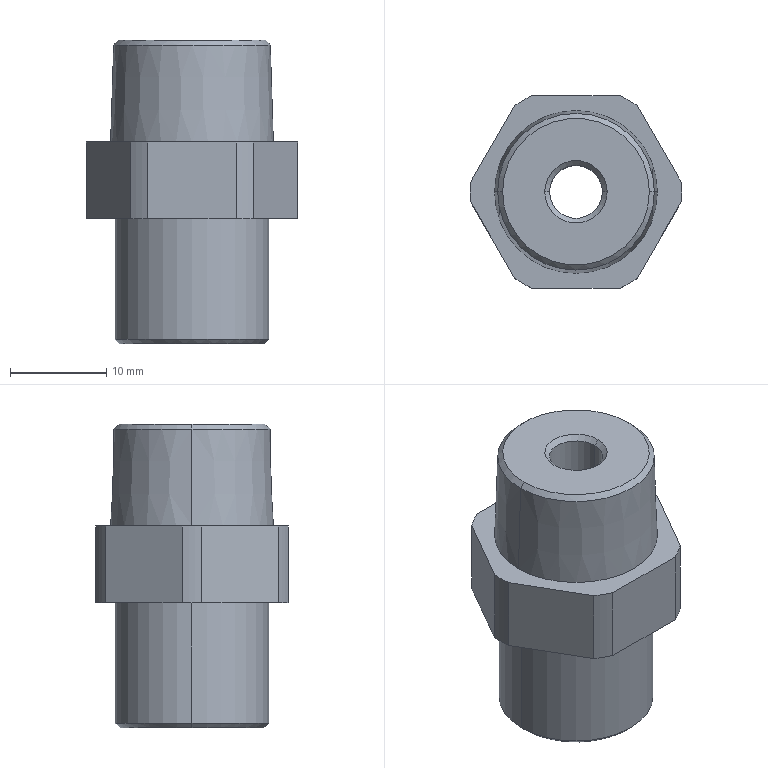Part | STEP file | HXGR200008-06-03-03 | 1 solid | 31 faces | box 22 x 20 x 31.6 mm | volume 6624 mm3 | cylinder 11 | cone 10 | plane 10 | commonest cylinder face diameters 22 x7 5.5 x2 16 x2
STEP:
#1=CARTESIAN_POINT('',(10.952,-1.031,0.));
#2=VERTEX_POINT('',#1);
#3=CARTESIAN_POINT('',(11.,0.,0.));
#4=VERTEX_POINT('',#3);
#5=CARTESIAN_POINT('',(0.,0.,0.));
#6=DIRECTION('',(0.,0.,1.));
#7=DIRECTION('',(1.,0.,0.));
#8=AXIS2_PLACEMENT_3D('',#5,#6,#7);
#9=CIRCLE('',#8,11.);
#10=EDGE_CURVE('',#2,#4,#9,.T.);
#11=ORIENTED_EDGE('',*,*,#10,.T.);
#12=CARTESIAN_POINT('',(11.,0.,8.));
#13=VERTEX_POINT('',#12);
#14=CARTESIAN_POINT('',(11.,0.,-13.));
#15=DIRECTION('',(0.,0.,1.));
#16=VECTOR('',#15,1000.);
#17=LINE('',#14,#16);
#18=EDGE_CURVE('',#4,#13,#17,.T.);
#19=ORIENTED_EDGE('',*,*,#18,.T.);
#20=CARTESIAN_POINT('',(10.952,-1.031,8.));
#21=VERTEX_POINT('',#20);
#22=CARTESIAN_POINT('',(0.,0.,8.));
#23=DIRECTION('',(0.,0.,1.));
#24=DIRECTION('',(1.,0.,0.));
#25=AXIS2_PLACEMENT_3D('',#22,#23,#24);
#26=CIRCLE('',#25,11.);
#27=EDGE_CURVE('',#21,#13,#26,.T.);
#28=ORIENTED_EDGE('',*,*,#27,.F.);
#29=CARTESIAN_POINT('',(10.952,-1.031,-13.));
#30=DIRECTION('',(0.,0.,-1.));
#31=VECTOR('',#30,1000.);
#32=LINE('',#29,#31);
#33=EDGE_CURVE('',#21,#2,#32,.T.);
#34=ORIENTED_EDGE('',*,*,#33,.T.);
#35=EDGE_LOOP('',(#11,#19,#28,#34));
#36=FACE_OUTER_BOUND('',#35,.T.);
#37=CARTESIAN_POINT('',(0.,0.,-13.));
#38=DIRECTION('',(0.,0.,1.));
#39=DIRECTION('',(1.,0.,0.));
#40=AXIS2_PLACEMENT_3D('',#37,#38,#39);
#41=CYLINDRICAL_SURFACE('',#40,11.);
#42=ADVANCED_FACE('',(#36),#41,.T.);
#43=CARTESIAN_POINT('',(-7.5,0.,-13.));
#44=VERTEX_POINT('',#43);
#45=CARTESIAN_POINT('',(7.5,0.,-13.));
#46=VERTEX_POINT('',#45);
#47=CARTESIAN_POINT('',(0.,0.,-13.));
#48=DIRECTION('',(0.,0.,-1.));
#49=DIRECTION('',(-1.,0.,0.));
#50=AXIS2_PLACEMENT_3D('',#47,#48,#49);
#51=CIRCLE('',#50,7.5);
#52=EDGE_CURVE('',#44,#46,#51,.T.);
#53=ORIENTED_EDGE('',*,*,#52,.F.);
#54=CARTESIAN_POINT('',(-8.,0.,-12.5));
#55=VERTEX_POINT('',#54);
#56=CARTESIAN_POINT('',(-7.5,0.,-13.));
#57=DIRECTION('',(-0.7071,0.,0.7071));
#58=VECTOR('',#57,1000.);
#59=LINE('',#56,#58);
#60=EDGE_CURVE('',#44,#55,#59,.T.);
#61=ORIENTED_EDGE('',*,*,#60,.T.);
#62=CARTESIAN_POINT('',(8.,0.,-12.5));
#63=VERTEX_POINT('',#62);
#64=CARTESIAN_POINT('',(0.,0.,-12.5));
#65=DIRECTION('',(0.,0.,1.));
#66=DIRECTION('',(-1.,0.,0.));
#67=AXIS2_PLACEMENT_3D('',#64,#65,#66);
#68=CIRCLE('',#67,8.);
#69=EDGE_CURVE('',#63,#55,#68,.T.);
#70=ORIENTED_EDGE('',*,*,#69,.F.);
#71=CARTESIAN_POINT('',(7.5,0.,-13.));
#72=DIRECTION('',(0.7071,0.,0.7071));
#73=VECTOR('',#72,1000.);
#74=LINE('',#71,#73);
#75=EDGE_CURVE('',#46,#63,#74,.T.);
#76=ORIENTED_EDGE('',*,*,#75,.F.);
#77=EDGE_LOOP('',(#53,#61,#70,#76));
#78=FACE_OUTER_BOUND('',#77,.T.);
#79=CARTESIAN_POINT('',(0.,0.,-13.));
#80=DIRECTION('',(0.,0.,1.));
#81=DIRECTION('',(1.,0.,0.));
#82=AXIS2_PLACEMENT_3D('',#79,#80,#81);
#83=CONICAL_SURFACE('',#82,7.5,0.7854);
#84=ADVANCED_FACE('',(#78),#83,.T.);
#85=CARTESIAN_POINT('',(7.63,0.,18.6));
#86=VERTEX_POINT('',#85);
#87=CARTESIAN_POINT('',(-7.63,0.,18.6));
#88=VERTEX_POINT('',#87);
#89=CARTESIAN_POINT('',(0.,0.,18.6));
#90=DIRECTION('',(0.,0.,1.));
#91=DIRECTION('',(1.,0.,0.));
#92=AXIS2_PLACEMENT_3D('',#89,#90,#91);
#93=CIRCLE('',#92,7.63);
#94=EDGE_CURVE('',#86,#88,#93,.T.);
#95=ORIENTED_EDGE('',*,*,#94,.F.);
#96=CARTESIAN_POINT('',(8.146,0.,18.084));
#97=VERTEX_POINT('',#96);
#98=CARTESIAN_POINT('',(8.146,0.,18.084));
#99=DIRECTION('',(0.7071,0.,-0.7071));
#100=VECTOR('',#99,1000.);
#101=LINE('',#98,#100);
#102=EDGE_CURVE('',#86,#97,#101,.T.);
#103=ORIENTED_EDGE('',*,*,#102,.T.);
#104=CARTESIAN_POINT('',(-8.146,0.,18.084));
#105=VERTEX_POINT('',#104);
#106=CARTESIAN_POINT('',(0.,0.,18.084));
#107=DIRECTION('',(0.,0.,-1.));
#108=DIRECTION('',(1.,0.,0.));
#109=AXIS2_PLACEMENT_3D('',#106,#107,#108);
#110=CIRCLE('',#109,8.146);
#111=EDGE_CURVE('',#105,#97,#110,.T.);
#112=ORIENTED_EDGE('',*,*,#111,.F.);
#113=CARTESIAN_POINT('',(-8.146,0.,18.084));
#114=DIRECTION('',(-0.7071,0.,-0.7071));
#115=VECTOR('',#114,1000.);
#116=LINE('',#113,#115);
#117=EDGE_CURVE('',#88,#105,#116,.T.);
#118=ORIENTED_EDGE('',*,*,#117,.F.);
#119=EDGE_LOOP('',(#95,#103,#112,#118));
#120=FACE_OUTER_BOUND('',#119,.T.);
#121=CARTESIAN_POINT('',(0.,0.,18.084));
#122=DIRECTION('',(0.,0.,-1.));
#123=DIRECTION('',(-1.,0.,0.));
#124=AXIS2_PLACEMENT_3D('',#121,#122,#123);
#125=CONICAL_SURFACE('',#124,8.146,0.7854);
#126=ADVANCED_FACE('',(#120),#125,.T.);
#127=CARTESIAN_POINT('',(-2.75,0.,18.1));
#128=VERTEX_POINT('',#127);
#129=CARTESIAN_POINT('',(2.75,0.,18.1));
#130=VERTEX_POINT('',#129);
#131=CARTESIAN_POINT('',(0.,0.,18.1));
#132=DIRECTION('',(0.,0.,1.));
#133=DIRECTION('',(1.,0.,0.));
#134=AXIS2_PLACEMENT_3D('',#131,#132,#133);
#135=CIRCLE('',#134,2.75);
#136=EDGE_CURVE('',#128,#130,#135,.T.);
#137=ORIENTED_EDGE('',*,*,#136,.F.);
#138=CARTESIAN_POINT('',(-3.25,0.,18.6));
#139=VERTEX_POINT('',#138);
#140=CARTESIAN_POINT('',(-2.75,0.,18.1));
#141=DIRECTION('',(-0.7071,0.,0.7071));
#142=VECTOR('',#141,1000.);
#143=LINE('',#140,#142);
#144=EDGE_CURVE('',#128,#139,#143,.T.);
#145=ORIENTED_EDGE('',*,*,#144,.T.);
#146=CARTESIAN_POINT('',(3.25,0.,18.6));
#147=VERTEX_POINT('',#146);
#148=CARTESIAN_POINT('',(0.,0.,18.6));
#149=DIRECTION('',(0.,0.,-1.));
#150=DIRECTION('',(1.,0.,0.));
#151=AXIS2_PLACEMENT_3D('',#148,#149,#150);
#152=CIRCLE('',#151,3.25);
#153=EDGE_CURVE('',#147,#139,#152,.T.);
#154=ORIENTED_EDGE('',*,*,#153,.F.);
#155=CARTESIAN_POINT('',(2.75,0.,18.1));
#156=DIRECTION('',(0.7071,0.,0.7071));
#157=VECTOR('',#156,1000.);
#158=LINE('',#155,#157);
#159=EDGE_CURVE('',#130,#147,#158,.T.);
#160=ORIENTED_EDGE('',*,*,#159,.F.);
#161=EDGE_LOOP('',(#137,#145,#154,#160));
#162=FACE_OUTER_BOUND('',#161,.T.);
#163=CARTESIAN_POINT('',(0.,0.,18.1));
#164=DIRECTION('',(0.,0.,1.));
#165=DIRECTION('',(1.,0.,0.));
#166=AXIS2_PLACEMENT_3D('',#163,#164,#165);
#167=CONICAL_SURFACE('',#166,2.75,0.7854);
#168=ADVANCED_FACE('',(#162),#167,.F.);
#169=CARTESIAN_POINT('',(2.75,0.,-6.938));
#170=VERTEX_POINT('',#169);
#171=CARTESIAN_POINT('',(-2.75,0.,-6.938));
#172=VERTEX_POINT('',#171);
#173=CARTESIAN_POINT('',(0.,0.,-6.938));
#174=DIRECTION('',(0.,0.,-1.));
#175=DIRECTION('',(-1.,0.,0.));
#176=AXIS2_PLACEMENT_3D('',#173,#174,#175);
#177=CIRCLE('',#176,2.75);
#178=EDGE_CURVE('',#170,#172,#177,.T.);
#179=ORIENTED_EDGE('',*,*,#178,.F.);
#180=CARTESIAN_POINT('',(6.25,0.,-13.));
#181=VERTEX_POINT('',#180);
#182=CARTESIAN_POINT('',(6.25,0.,-13.));
#183=DIRECTION('',(0.5,0.,-0.866));
#184=VECTOR('',#183,1000.);
#185=LINE('',#182,#184);
#186=EDGE_CURVE('',#170,#181,#185,.T.);
#187=ORIENTED_EDGE('',*,*,#186,.T.);
#188=CARTESIAN_POINT('',(-6.25,0.,-13.));
#189=VERTEX_POINT('',#188);
#190=CARTESIAN_POINT('',(0.,0.,-13.));
#191=DIRECTION('',(0.,0.,-1.));
#192=DIRECTION('',(-1.,0.,0.));
#193=AXIS2_PLACEMENT_3D('',#190,#191,#192);
#194=CIRCLE('',#193,6.25);
#195=EDGE_CURVE('',#181,#189,#194,.T.);
#196=ORIENTED_EDGE('',*,*,#195,.T.);
#197=CARTESIAN_POINT('',(-6.25,0.,-13.));
#198=DIRECTION('',(-0.5,0.,-0.866));
#199=VECTOR('',#198,1000.);
#200=LINE('',#197,#199);
#201=EDGE_CURVE('',#172,#189,#200,.T.);
#202=ORIENTED_EDGE('',*,*,#201,.F.);
#203=EDGE_LOOP('',(#179,#187,#196,#202));
#204=FACE_OUTER_BOUND('',#203,.T.);
#205=CARTESIAN_POINT('',(0.,0.,-13.));
#206=DIRECTION('',(0.,0.,-1.));
#207=DIRECTION('',(-1.,0.,0.));
#208=AXIS2_PLACEMENT_3D('',#205,#206,#207);
#209=CONICAL_SURFACE('',#208,6.25,0.5236);
#210=ADVANCED_FACE('',(#204),#209,.F.);
#211=ORIENTED_EDGE('',*,*,#178,.T.);
#212=CARTESIAN_POINT('',(-2.75,0.,-13.001));
#213=DIRECTION('',(0.,0.,1.));
#214=VECTOR('',#213,1000.);
#215=LINE('',#212,#214);
#216=EDGE_CURVE('',#172,#128,#215,.T.);
#217=ORIENTED_EDGE('',*,*,#216,.T.);
#218=ORIENTED_EDGE('',*,*,#136,.T.);
#219=CARTESIAN_POINT('',(2.75,0.,-13.001));
#220=DIRECTION('',(0.,0.,1.));
#221=VECTOR('',#220,1000.);
#222=LINE('',#219,#221);
#223=EDGE_CURVE('',#170,#130,#222,.T.);
#224=ORIENTED_EDGE('',*,*,#223,.F.);
#225=EDGE_LOOP('',(#211,#217,#218,#224));
#226=FACE_OUTER_BOUND('',#225,.T.);
#227=CARTESIAN_POINT('',(0.,0.,-13.001));
#228=DIRECTION('',(0.,0.,1.));
#229=DIRECTION('',(1.,0.,0.));
#230=AXIS2_PLACEMENT_3D('',#227,#228,#229);
#231=CYLINDRICAL_SURFACE('',#230,2.75);
#232=ADVANCED_FACE('',(#226),#231,.F.);
#233=ORIENTED_EDGE('',*,*,#111,.T.);
#234=CARTESIAN_POINT('',(8.46,0.,8.));
#235=VERTEX_POINT('',#234);
#236=CARTESIAN_POINT('',(8.46,0.,8.));
#237=DIRECTION('',(0.03112,0.,-0.9995));
#238=VECTOR('',#237,1000.);
#239=LINE('',#236,#238);
#240=EDGE_CURVE('',#97,#235,#239,.T.);
#241=ORIENTED_EDGE('',*,*,#240,.T.);
#242=CARTESIAN_POINT('',(-8.46,0.,8.));
#243=VERTEX_POINT('',#242);
#244=CARTESIAN_POINT('',(0.,0.,8.));
#245=DIRECTION('',(0.,0.,-1.));
#246=DIRECTION('',(-1.,0.,0.));
#247=AXIS2_PLACEMENT_3D('',#244,#245,#246);
#248=CIRCLE('',#247,8.46);
#249=EDGE_CURVE('',#243,#235,#248,.T.);
#250=ORIENTED_EDGE('',*,*,#249,.F.);
#251=CARTESIAN_POINT('',(-8.46,0.,8.));
#252=DIRECTION('',(-0.03112,0.,-0.9995));
#253=VECTOR('',#252,1000.);
#254=LINE('',#251,#253);
#255=EDGE_CURVE('',#105,#243,#254,.T.);
#256=ORIENTED_EDGE('',*,*,#255,.F.);
#257=EDGE_LOOP('',(#233,#241,#250,#256));
#258=FACE_OUTER_BOUND('',#257,.T.);
#259=CARTESIAN_POINT('',(0.,0.,8.));
#260=DIRECTION('',(0.,0.,-1.));
#261=DIRECTION('',(-1.,0.,0.));
#262=AXIS2_PLACEMENT_3D('',#259,#260,#261);
#263=CONICAL_SURFACE('',#262,8.46,0.03112);
#264=ADVANCED_FACE('',(#258),#263,.T.);
#265=ORIENTED_EDGE('',*,*,#69,.T.);
#266=CARTESIAN_POINT('',(-8.,0.,0.));
#267=VERTEX_POINT('',#266);
#268=CARTESIAN_POINT('',(-8.,0.,-13.));
#269=DIRECTION('',(0.,0.,1.));
#270=VECTOR('',#269,1000.);
#271=LINE('',#268,#270);
#272=EDGE_CURVE('',#55,#267,#271,.T.);
#273=ORIENTED_EDGE('',*,*,#272,.T.);
#274=CARTESIAN_POINT('',(8.,0.,0.));
#275=VERTEX_POINT('',#274);
#276=CARTESIAN_POINT('',(0.,0.,0.));
#277=DIRECTION('',(0.,0.,-1.));
#278=DIRECTION('',(-1.,0.,0.));
#279=AXIS2_PLACEMENT_3D('',#276,#277,#278);
#280=CIRCLE('',#279,8.);
#281=EDGE_CURVE('',#267,#275,#280,.T.);
#282=ORIENTED_EDGE('',*,*,#281,.T.);
#283=CARTESIAN_POINT('',(8.,0.,-13.));
#284=DIRECTION('',(0.,0.,1.));
#285=VECTOR('',#284,1000.);
#286=LINE('',#283,#285);
#287=EDGE_CURVE('',#63,#275,#286,.T.);
#288=ORIENTED_EDGE('',*,*,#287,.F.);
#289=EDGE_LOOP('',(#265,#273,#282,#288));
#290=FACE_OUTER_BOUND('',#289,.T.);
#291=CARTESIAN_POINT('',(0.,0.,-13.));
#292=DIRECTION('',(0.,0.,1.));
#293=DIRECTION('',(1.,0.,0.));
#294=AXIS2_PLACEMENT_3D('',#291,#292,#293);
#295=CYLINDRICAL_SURFACE('',#294,8.);
#296=ADVANCED_FACE('',(#290),#295,.T.);
#297=CARTESIAN_POINT('',(6.369,-8.969,0.));
#298=VERTEX_POINT('',#297);
#299=CARTESIAN_POINT('',(6.369,-8.969,8.));
#300=VERTEX_POINT('',#299);
#301=CARTESIAN_POINT('',(6.369,-8.969,-13.));
#302=DIRECTION('',(0.,0.,1.));
#303=VECTOR('',#302,1000.);
#304=LINE('',#301,#303);
#305=EDGE_CURVE('',#298,#300,#304,.T.);
#306=ORIENTED_EDGE('',*,*,#305,.F.);
#307=CARTESIAN_POINT('',(5.774,-10.,0.));
#308=DIRECTION('',(0.5,0.866,0.));
#309=VECTOR('',#308,1000.);
#310=LINE('',#307,#309);
#311=EDGE_CURVE('',#298,#2,#310,.T.);
#312=ORIENTED_EDGE('',*,*,#311,.T.);
#313=ORIENTED_EDGE('',*,*,#33,.F.);
#314=CARTESIAN_POINT('',(5.774,-10.,8.));
#315=DIRECTION('',(0.5,0.866,0.));
#316=VECTOR('',#315,1000.);
#317=LINE('',#314,#316);
#318=EDGE_CURVE('',#300,#21,#317,.T.);
#319=ORIENTED_EDGE('',*,*,#318,.F.);
#320=EDGE_LOOP('',(#306,#312,#313,#319));
#321=FACE_OUTER_BOUND('',#320,.T.);
#322=CARTESIAN_POINT('',(5.774,-10.,8.));
#323=DIRECTION('',(-0.866,0.5,0.));
#324=DIRECTION('',(-0.5,-0.866,0.));
#325=AXIS2_PLACEMENT_3D('',#322,#323,#324);
#326=PLANE('',#325);
#327=ADVANCED_FACE('',(#321),#326,.F.);
#328=CARTESIAN_POINT('',(10.952,1.031,0.));
#329=VERTEX_POINT('',#328);
#330=CARTESIAN_POINT('',(10.952,1.031,8.));
#331=VERTEX_POINT('',#330);
#332=CARTESIAN_POINT('',(10.952,1.031,-13.));
#333=DIRECTION('',(0.,0.,1.));
#334=VECTOR('',#333,1000.);
#335=LINE('',#332,#334);
#336=EDGE_CURVE('',#329,#331,#335,.T.);
#337=ORIENTED_EDGE('',*,*,#336,.F.);
#338=CARTESIAN_POINT('',(6.369,8.969,0.));
#339=VERTEX_POINT('',#338);
#340=CARTESIAN_POINT('',(11.547,0.,0.));
#341=DIRECTION('',(-0.5,0.866,0.));
#342=VECTOR('',#341,1000.);
#343=LINE('',#340,#342);
#344=EDGE_CURVE('',#329,#339,#343,.T.);
#345=ORIENTED_EDGE('',*,*,#344,.T.);
#346=CARTESIAN_POINT('',(6.369,8.969,8.));
#347=VERTEX_POINT('',#346);
#348=CARTESIAN_POINT('',(6.369,8.969,-13.));
#349=DIRECTION('',(0.,0.,-1.));
#350=VECTOR('',#349,1000.);
#351=LINE('',#348,#350);
#352=EDGE_CURVE('',#347,#339,#351,.T.);
#353=ORIENTED_EDGE('',*,*,#352,.F.);
#354=CARTESIAN_POINT('',(11.547,0.,8.));
#355=DIRECTION('',(-0.5,0.866,0.));
#356=VECTOR('',#355,1000.);
#357=LINE('',#354,#356);
#358=EDGE_CURVE('',#331,#347,#357,.T.);
#359=ORIENTED_EDGE('',*,*,#358,.F.);
#360=EDGE_LOOP('',(#337,#345,#353,#359));
#361=FACE_OUTER_BOUND('',#360,.T.);
#362=CARTESIAN_POINT('',(11.547,0.,8.));
#363=DIRECTION('',(-0.866,-0.5,0.));
#364=DIRECTION('',(0.5,-0.866,0.));
#365=AXIS2_PLACEMENT_3D('',#362,#363,#364);
#366=PLANE('',#365);
#367=ADVANCED_FACE('',(#361),#366,.F.);
#368=CARTESIAN_POINT('',(4.583,10.,0.));
#369=VERTEX_POINT('',#368);
#370=CARTESIAN_POINT('',(4.583,10.,8.));
#371=VERTEX_POINT('',#370);
#372=CARTESIAN_POINT('',(4.583,10.,-13.));
#373=DIRECTION('',(0.,0.,1.));
#374=VECTOR('',#373,1000.);
#375=LINE('',#372,#374);
#376=EDGE_CURVE('',#369,#371,#375,.T.);
#377=ORIENTED_EDGE('',*,*,#376,.F.);
#378=CARTESIAN_POINT('',(-4.583,10.,0.));
#379=VERTEX_POINT('',#378);
#380=CARTESIAN_POINT('',(5.774,10.,0.));
#381=DIRECTION('',(-1.,0.,0.));
#382=VECTOR('',#381,1000.);
#383=LINE('',#380,#382);
#384=EDGE_CURVE('',#369,#379,#383,.T.);
#385=ORIENTED_EDGE('',*,*,#384,.T.);
#386=CARTESIAN_POINT('',(-4.583,10.,8.));
#387=VERTEX_POINT('',#386);
#388=CARTESIAN_POINT('',(-4.583,10.,-13.));
#389=DIRECTION('',(0.,0.,-1.));
#390=VECTOR('',#389,1000.);
#391=LINE('',#388,#390);
#392=EDGE_CURVE('',#387,#379,#391,.T.);
#393=ORIENTED_EDGE('',*,*,#392,.F.);
#394=CARTESIAN_POINT('',(5.774,10.,8.));
#395=DIRECTION('',(-1.,0.,0.));
#396=VECTOR('',#395,1000.);
#397=LINE('',#394,#396);
#398=EDGE_CURVE('',#371,#387,#397,.T.);
#399=ORIENTED_EDGE('',*,*,#398,.F.);
#400=EDGE_LOOP('',(#377,#385,#393,#399));
#401=FACE_OUTER_BOUND('',#400,.T.);
#402=CARTESIAN_POINT('',(5.774,10.,8.));
#403=DIRECTION('',(0.,-1.,0.));
#404=DIRECTION('',(1.,0.,0.));
#405=AXIS2_PLACEMENT_3D('',#402,#403,#404);
#406=PLANE('',#405);
#407=ADVANCED_FACE('',(#401),#406,.F.);
#408=CARTESIAN_POINT('',(-6.369,8.969,0.));
#409=VERTEX_POINT('',#408);
#410=CARTESIAN_POINT('',(-6.369,8.969,8.));
#411=VERTEX_POINT('',#410);
#412=CARTESIAN_POINT('',(-6.369,8.969,-13.));
#413=DIRECTION('',(0.,0.,1.));
#414=VECTOR('',#413,1000.);
#415=LINE('',#412,#414);
#416=EDGE_CURVE('',#409,#411,#415,.T.);
#417=ORIENTED_EDGE('',*,*,#416,.F.);
#418=CARTESIAN_POINT('',(-10.952,1.031,0.));
#419=VERTEX_POINT('',#418);
#420=CARTESIAN_POINT('',(-5.774,10.,0.));
#421=DIRECTION('',(-0.5,-0.866,0.));
#422=VECTOR('',#421,1000.);
#423=LINE('',#420,#422);
#424=EDGE_CURVE('',#409,#419,#423,.T.);
#425=ORIENTED_EDGE('',*,*,#424,.T.);
#426=CARTESIAN_POINT('',(-10.952,1.031,8.));
#427=VERTEX_POINT('',#426);
#428=CARTESIAN_POINT('',(-10.952,1.031,-13.));
#429=DIRECTION('',(0.,0.,-1.));
#430=VECTOR('',#429,1000.);
#431=LINE('',#428,#430);
#432=EDGE_CURVE('',#427,#419,#431,.T.);
#433=ORIENTED_EDGE('',*,*,#432,.F.);
#434=CARTESIAN_POINT('',(-5.774,10.,8.));
#435=DIRECTION('',(-0.5,-0.866,0.));
#436=VECTOR('',#435,1000.);
#437=LINE('',#434,#436);
#438=EDGE_CURVE('',#411,#427,#437,.T.);
#439=ORIENTED_EDGE('',*,*,#438,.F.);
#440=EDGE_LOOP('',(#417,#425,#433,#439));
#441=FACE_OUTER_BOUND('',#440,.T.);
#442=CARTESIAN_POINT('',(-5.774,10.,8.));
#443=DIRECTION('',(0.866,-0.5,0.));
#444=DIRECTION('',(0.5,0.866,0.));
#445=AXIS2_PLACEMENT_3D('',#442,#443,#444);
#446=PLANE('',#445);
#447=ADVANCED_FACE('',(#441),#446,.F.);
#448=CARTESIAN_POINT('',(-10.952,-1.031,0.));
#449=VERTEX_POINT('',#448);
#450=CARTESIAN_POINT('',(-10.952,-1.031,8.));
#451=VERTEX_POINT('',#450);
#452=CARTESIAN_POINT('',(-10.952,-1.031,-13.));
#453=DIRECTION('',(0.,0.,1.));
#454=VECTOR('',#453,1000.);
#455=LINE('',#452,#454);
#456=EDGE_CURVE('',#449,#451,#455,.T.);
#457=ORIENTED_EDGE('',*,*,#456,.F.);
#458=CARTESIAN_POINT('',(-6.369,-8.969,0.));
#459=VERTEX_POINT('',#458);
#460=CARTESIAN_POINT('',(-11.547,0.,0.));
#461=DIRECTION('',(0.5,-0.866,0.));
#462=VECTOR('',#461,1000.);
#463=LINE('',#460,#462);
#464=EDGE_CURVE('',#449,#459,#463,.T.);
#465=ORIENTED_EDGE('',*,*,#464,.T.);
#466=CARTESIAN_POINT('',(-6.369,-8.969,8.));
#467=VERTEX_POINT('',#466);
#468=CARTESIAN_POINT('',(-6.369,-8.969,-13.));
#469=DIRECTION('',(0.,0.,-1.));
#470=VECTOR('',#469,1000.);
#471=LINE('',#468,#470);
#472=EDGE_CURVE('',#467,#459,#471,.T.);
#473=ORIENTED_EDGE('',*,*,#472,.F.);
#474=CARTESIAN_POINT('',(-11.547,0.,8.));
#475=DIRECTION('',(0.5,-0.866,0.));
#476=VECTOR('',#475,1000.);
#477=LINE('',#474,#476);
#478=EDGE_CURVE('',#451,#467,#477,.T.);
#479=ORIENTED_EDGE('',*,*,#478,.F.);
#480=EDGE_LOOP('',(#457,#465,#473,#479));
#481=FACE_OUTER_BOUND('',#480,.T.);
#482=CARTESIAN_POINT('',(-11.547,0.,8.));
#483=DIRECTION('',(0.866,0.5,0.));
#484=DIRECTION('',(-0.5,0.866,0.));
#485=AXIS2_PLACEMENT_3D('',#482,#483,#484);
#486=PLANE('',#485);
#487=ADVANCED_FACE('',(#481),#486,.F.);
#488=CARTESIAN_POINT('',(-4.583,-10.,0.));
#489=VERTEX_POINT('',#488);
#490=CARTESIAN_POINT('',(-4.583,-10.,8.));
#491=VERTEX_POINT('',#490);
#492=CARTESIAN_POINT('',(-4.583,-10.,-13.));
#493=DIRECTION('',(0.,0.,1.));
#494=VECTOR('',#493,1000.);
#495=LINE('',#492,#494);
#496=EDGE_CURVE('',#489,#491,#495,.T.);
#497=ORIENTED_EDGE('',*,*,#496,.F.);
#498=CARTESIAN_POINT('',(4.583,-10.,0.));
#499=VERTEX_POINT('',#498);
#500=CARTESIAN_POINT('',(-5.774,-10.,0.));
#501=DIRECTION('',(1.,0.,0.));
#502=VECTOR('',#501,1000.);
#503=LINE('',#500,#502);
#504=EDGE_CURVE('',#489,#499,#503,.T.);
#505=ORIENTED_EDGE('',*,*,#504,.T.);
#506=CARTESIAN_POINT('',(4.583,-10.,8.));
#507=VERTEX_POINT('',#506);
#508=CARTESIAN_POINT('',(4.583,-10.,-13.));
#509=DIRECTION('',(0.,0.,-1.));
#510=VECTOR('',#509,1000.);
#511=LINE('',#508,#510);
#512=EDGE_CURVE('',#507,#499,#511,.T.);
#513=ORIENTED_EDGE('',*,*,#512,.F.);
#514=CARTESIAN_POINT('',(-5.774,-10.,8.));
#515=DIRECTION('',(1.,0.,0.));
#516=VECTOR('',#515,1000.);
#517=LINE('',#514,#516);
#518=EDGE_CURVE('',#491,#507,#517,.T.);
#519=ORIENTED_EDGE('',*,*,#518,.F.);
#520=EDGE_LOOP('',(#497,#505,#513,#519));
#521=FACE_OUTER_BOUND('',#520,.T.);
#522=CARTESIAN_POINT('',(-5.774,-10.,8.));
#523=DIRECTION('',(0.,1.,0.));
#524=DIRECTION('',(-1.,0.,0.));
#525=AXIS2_PLACEMENT_3D('',#522,#523,#524);
#526=PLANE('',#525);
#527=ADVANCED_FACE('',(#521),#526,.F.);
#528=ORIENTED_EDGE('',*,*,#249,.T.);
#529=CARTESIAN_POINT('',(0.,0.,8.));
#530=DIRECTION('',(0.,0.,-1.));
#531=DIRECTION('',(-1.,0.,0.));
#532=AXIS2_PLACEMENT_3D('',#529,#530,#531);
#533=CIRCLE('',#532,8.46);
#534=EDGE_CURVE('',#235,#243,#533,.T.);
#535=ORIENTED_EDGE('',*,*,#534,.T.);
#536=EDGE_LOOP('',(#528,#535));
#537=FACE_BOUND('',#536,.T.);
#538=ORIENTED_EDGE('',*,*,#358,.T.);
#539=CARTESIAN_POINT('',(0.,0.,8.));
#540=DIRECTION('',(0.,0.,1.));
#541=DIRECTION('',(1.,0.,0.));
#542=AXIS2_PLACEMENT_3D('',#539,#540,#541);
#543=CIRCLE('',#542,11.);
#544=EDGE_CURVE('',#347,#371,#543,.T.);
#545=ORIENTED_EDGE('',*,*,#544,.T.);
#546=ORIENTED_EDGE('',*,*,#398,.T.);
#547=CARTESIAN_POINT('',(0.,0.,8.));
#548=DIRECTION('',(0.,0.,1.));
#549=DIRECTION('',(1.,0.,0.));
#550=AXIS2_PLACEMENT_3D('',#547,#548,#549);
#551=CIRCLE('',#550,11.);
#552=EDGE_CURVE('',#387,#411,#551,.T.);
#553=ORIENTED_EDGE('',*,*,#552,.T.);
#554=ORIENTED_EDGE('',*,*,#438,.T.);
#555=CARTESIAN_POINT('',(0.,0.,8.));
#556=DIRECTION('',(0.,0.,1.));
#557=DIRECTION('',(1.,0.,0.));
#558=AXIS2_PLACEMENT_3D('',#555,#556,#557);
#559=CIRCLE('',#558,11.);
#560=EDGE_CURVE('',#427,#451,#559,.T.);
#561=ORIENTED_EDGE('',*,*,#560,.T.);
#562=ORIENTED_EDGE('',*,*,#478,.T.);
#563=CARTESIAN_POINT('',(0.,0.,8.));
#564=DIRECTION('',(0.,0.,1.));
#565=DIRECTION('',(1.,0.,0.));
#566=AXIS2_PLACEMENT_3D('',#563,#564,#565);
#567=CIRCLE('',#566,11.);
#568=EDGE_CURVE('',#467,#491,#567,.T.);
#569=ORIENTED_EDGE('',*,*,#568,.T.);
#570=ORIENTED_EDGE('',*,*,#518,.T.);
#571=CARTESIAN_POINT('',(0.,0.,8.));
#572=DIRECTION('',(0.,0.,1.));
#573=DIRECTION('',(1.,0.,0.));
#574=AXIS2_PLACEMENT_3D('',#571,#572,#573);
#575=CIRCLE('',#574,11.);
#576=EDGE_CURVE('',#507,#300,#575,.T.);
#577=ORIENTED_EDGE('',*,*,#576,.T.);
#578=ORIENTED_EDGE('',*,*,#318,.T.);
#579=ORIENTED_EDGE('',*,*,#27,.T.);
#580=CARTESIAN_POINT('',(0.,0.,8.));
#581=DIRECTION('',(0.,0.,1.));
#582=DIRECTION('',(1.,0.,0.));
#583=AXIS2_PLACEMENT_3D('',#580,#581,#582);
#584=CIRCLE('',#583,11.);
#585=EDGE_CURVE('',#13,#331,#584,.T.);
#586=ORIENTED_EDGE('',*,*,#585,.T.);
#587=EDGE_LOOP('',(#538,#545,#546,#553,#554,#561,#562,#569,#570,#577,#578,#579,#586));
#588=FACE_OUTER_BOUND('',#587,.T.);
#589=CARTESIAN_POINT('',(0.,0.,8.));
#590=DIRECTION('',(0.,0.,1.));
#591=DIRECTION('',(1.,0.,0.));
#592=AXIS2_PLACEMENT_3D('',#589,#590,#591);
#593=PLANE('',#592);
#594=ADVANCED_FACE('',(#537,#588),#593,.T.);
#595=CARTESIAN_POINT('',(0.,0.,0.));
#596=DIRECTION('',(0.,0.,-1.));
#597=DIRECTION('',(-1.,0.,0.));
#598=AXIS2_PLACEMENT_3D('',#595,#596,#597);
#599=CIRCLE('',#598,8.);
#600=EDGE_CURVE('',#275,#267,#599,.T.);
#601=ORIENTED_EDGE('',*,*,#600,.F.);
#602=ORIENTED_EDGE('',*,*,#281,.F.);
#603=EDGE_LOOP('',(#601,#602));
#604=FACE_BOUND('',#603,.T.);
#605=CARTESIAN_POINT('',(0.,0.,0.));
#606=DIRECTION('',(0.,0.,1.));
#607=DIRECTION('',(1.,0.,0.));
#608=AXIS2_PLACEMENT_3D('',#605,#606,#607);
#609=CIRCLE('',#608,11.);
#610=EDGE_CURVE('',#339,#369,#609,.T.);
#611=ORIENTED_EDGE('',*,*,#610,.F.);
#612=ORIENTED_EDGE('',*,*,#344,.F.);
#613=CARTESIAN_POINT('',(0.,0.,0.));
#614=DIRECTION('',(0.,0.,1.));
#615=DIRECTION('',(1.,0.,0.));
#616=AXIS2_PLACEMENT_3D('',#613,#614,#615);
#617=CIRCLE('',#616,11.);
#618=EDGE_CURVE('',#4,#329,#617,.T.);
#619=ORIENTED_EDGE('',*,*,#618,.F.);
#620=ORIENTED_EDGE('',*,*,#10,.F.);
#621=ORIENTED_EDGE('',*,*,#311,.F.);
#622=CARTESIAN_POINT('',(0.,0.,0.));
#623=DIRECTION('',(0.,0.,1.));
#624=DIRECTION('',(1.,0.,0.));
#625=AXIS2_PLACEMENT_3D('',#622,#623,#624);
#626=CIRCLE('',#625,11.);
#627=EDGE_CURVE('',#499,#298,#626,.T.);
#628=ORIENTED_EDGE('',*,*,#627,.F.);
#629=ORIENTED_EDGE('',*,*,#504,.F.);
#630=CARTESIAN_POINT('',(0.,0.,0.));
#631=DIRECTION('',(0.,0.,1.));
#632=DIRECTION('',(1.,0.,0.));
#633=AXIS2_PLACEMENT_3D('',#630,#631,#632);
#634=CIRCLE('',#633,11.);
#635=EDGE_CURVE('',#459,#489,#634,.T.);
#636=ORIENTED_EDGE('',*,*,#635,.F.);
#637=ORIENTED_EDGE('',*,*,#464,.F.);
#638=CARTESIAN_POINT('',(0.,0.,0.));
#639=DIRECTION('',(0.,0.,1.));
#640=DIRECTION('',(1.,0.,0.));
#641=AXIS2_PLACEMENT_3D('',#638,#639,#640);
#642=CIRCLE('',#641,11.);
#643=EDGE_CURVE('',#419,#449,#642,.T.);
#644=ORIENTED_EDGE('',*,*,#643,.F.);
#645=ORIENTED_EDGE('',*,*,#424,.F.);
#646=CARTESIAN_POINT('',(0.,0.,0.));
#647=DIRECTION('',(0.,0.,1.));
#648=DIRECTION('',(1.,0.,0.));
#649=AXIS2_PLACEMENT_3D('',#646,#647,#648);
#650=CIRCLE('',#649,11.);
#651=EDGE_CURVE('',#379,#409,#650,.T.);
#652=ORIENTED_EDGE('',*,*,#651,.F.);
#653=ORIENTED_EDGE('',*,*,#384,.F.);
#654=EDGE_LOOP('',(#611,#612,#619,#620,#621,#628,#629,#636,#637,#644,#645,#652,#653));
#655=FACE_OUTER_BOUND('',#654,.T.);
#656=CARTESIAN_POINT('',(0.,0.,0.));
#657=DIRECTION('',(0.,0.,1.));
#658=DIRECTION('',(1.,0.,0.));
#659=AXIS2_PLACEMENT_3D('',#656,#657,#658);
#660=PLANE('',#659);
#661=ADVANCED_FACE('',(#604,#655),#660,.F.);
#662=ORIENTED_EDGE('',*,*,#272,.F.);
#663=CARTESIAN_POINT('',(0.,0.,-12.5));
#664=DIRECTION('',(0.,0.,1.));
#665=DIRECTION('',(-1.,0.,0.));
#666=AXIS2_PLACEMENT_3D('',#663,#664,#665);
#667=CIRCLE('',#666,8.);
#668=EDGE_CURVE('',#55,#63,#667,.T.);
#669=ORIENTED_EDGE('',*,*,#668,.T.);
#670=ORIENTED_EDGE('',*,*,#287,.T.);
#671=ORIENTED_EDGE('',*,*,#600,.T.);
#672=EDGE_LOOP('',(#662,#669,#670,#671));
#673=FACE_OUTER_BOUND('',#672,.T.);
#674=CARTESIAN_POINT('',(0.,0.,-13.));
#675=DIRECTION('',(0.,0.,1.));
#676=DIRECTION('',(1.,0.,0.));
#677=AXIS2_PLACEMENT_3D('',#674,#675,#676);
#678=CYLINDRICAL_SURFACE('',#677,8.);
#679=ADVANCED_FACE('',(#673),#678,.T.);
#680=CARTESIAN_POINT('',(0.,0.,-13.));
#681=DIRECTION('',(0.,0.,-1.));
#682=DIRECTION('',(-1.,0.,0.));
#683=AXIS2_PLACEMENT_3D('',#680,#681,#682);
#684=CIRCLE('',#683,7.5);
#685=EDGE_CURVE('',#46,#44,#684,.T.);
#686=ORIENTED_EDGE('',*,*,#685,.T.);
#687=ORIENTED_EDGE('',*,*,#52,.T.);
#688=EDGE_LOOP('',(#686,#687));
#689=FACE_OUTER_BOUND('',#688,.T.);
#690=CARTESIAN_POINT('',(0.,0.,-13.));
#691=DIRECTION('',(0.,0.,-1.));
#692=DIRECTION('',(-1.,0.,0.));
#693=AXIS2_PLACEMENT_3D('',#690,#691,#692);
#694=CIRCLE('',#693,6.25);
#695=EDGE_CURVE('',#189,#181,#694,.T.);
#696=ORIENTED_EDGE('',*,*,#695,.F.);
#697=ORIENTED_EDGE('',*,*,#195,.F.);
#698=EDGE_LOOP('',(#696,#697));
#699=FACE_BOUND('',#698,.T.);
#700=CARTESIAN_POINT('',(0.,0.,-13.));
#701=DIRECTION('',(0.,0.,-1.));
#702=DIRECTION('',(-1.,0.,0.));
#703=AXIS2_PLACEMENT_3D('',#700,#701,#702);
#704=PLANE('',#703);
#705=ADVANCED_FACE('',(#689,#699),#704,.T.);
#706=ORIENTED_EDGE('',*,*,#153,.T.);
#707=CARTESIAN_POINT('',(0.,0.,18.6));
#708=DIRECTION('',(0.,0.,-1.));
#709=DIRECTION('',(1.,0.,0.));
#710=AXIS2_PLACEMENT_3D('',#707,#708,#709);
#711=CIRCLE('',#710,3.25);
#712=EDGE_CURVE('',#139,#147,#711,.T.);
#713=ORIENTED_EDGE('',*,*,#712,.T.);
#714=EDGE_LOOP('',(#706,#713));
#715=FACE_BOUND('',#714,.T.);
#716=CARTESIAN_POINT('',(0.,0.,18.6));
#717=DIRECTION('',(0.,0.,1.));
#718=DIRECTION('',(1.,0.,0.));
#719=AXIS2_PLACEMENT_3D('',#716,#717,#718);
#720=CIRCLE('',#719,7.63);
#721=EDGE_CURVE('',#88,#86,#720,.T.);
#722=ORIENTED_EDGE('',*,*,#721,.T.);
#723=ORIENTED_EDGE('',*,*,#94,.T.);
#724=EDGE_LOOP('',(#722,#723));
#725=FACE_OUTER_BOUND('',#724,.T.);
#726=CARTESIAN_POINT('',(0.,0.,18.6));
#727=DIRECTION('',(0.,0.,1.));
#728=DIRECTION('',(1.,0.,0.));
#729=AXIS2_PLACEMENT_3D('',#726,#727,#728);
#730=PLANE('',#729);
#731=ADVANCED_FACE('',(#715,#725),#730,.T.);
#732=ORIENTED_EDGE('',*,*,#240,.F.);
#733=CARTESIAN_POINT('',(0.,0.,18.084));
#734=DIRECTION('',(0.,0.,-1.));
#735=DIRECTION('',(1.,0.,0.));
#736=AXIS2_PLACEMENT_3D('',#733,#734,#735);
#737=CIRCLE('',#736,8.146);
#738=EDGE_CURVE('',#97,#105,#737,.T.);
#739=ORIENTED_EDGE('',*,*,#738,.T.);
#740=ORIENTED_EDGE('',*,*,#255,.T.);
#741=ORIENTED_EDGE('',*,*,#534,.F.);
#742=EDGE_LOOP('',(#732,#739,#740,#741));
#743=FACE_OUTER_BOUND('',#742,.T.);
#744=CARTESIAN_POINT('',(0.,0.,8.));
#745=DIRECTION('',(0.,0.,-1.));
#746=DIRECTION('',(-1.,0.,0.));
#747=AXIS2_PLACEMENT_3D('',#744,#745,#746);
#748=CONICAL_SURFACE('',#747,8.46,0.03112);
#749=ADVANCED_FACE('',(#743),#748,.T.);
#750=ORIENTED_EDGE('',*,*,#216,.F.);
#751=CARTESIAN_POINT('',(0.,0.,-6.938));
#752=DIRECTION('',(0.,0.,-1.));
#753=DIRECTION('',(-1.,0.,0.));
#754=AXIS2_PLACEMENT_3D('',#751,#752,#753);
#755=CIRCLE('',#754,2.75);
#756=EDGE_CURVE('',#172,#170,#755,.T.);
#757=ORIENTED_EDGE('',*,*,#756,.T.);
#758=ORIENTED_EDGE('',*,*,#223,.T.);
#759=CARTESIAN_POINT('',(0.,0.,18.1));
#760=DIRECTION('',(0.,0.,1.));
#761=DIRECTION('',(1.,0.,0.));
#762=AXIS2_PLACEMENT_3D('',#759,#760,#761);
#763=CIRCLE('',#762,2.75);
#764=EDGE_CURVE('',#130,#128,#763,.T.);
#765=ORIENTED_EDGE('',*,*,#764,.T.);
#766=EDGE_LOOP('',(#750,#757,#758,#765));
#767=FACE_OUTER_BOUND('',#766,.T.);
#768=CARTESIAN_POINT('',(0.,0.,-13.001));
#769=DIRECTION('',(0.,0.,1.));
#770=DIRECTION('',(1.,0.,0.));
#771=AXIS2_PLACEMENT_3D('',#768,#769,#770);
#772=CYLINDRICAL_SURFACE('',#771,2.75);
#773=ADVANCED_FACE('',(#767),#772,.F.);
#774=ORIENTED_EDGE('',*,*,#186,.F.);
#775=ORIENTED_EDGE('',*,*,#756,.F.);
#776=ORIENTED_EDGE('',*,*,#201,.T.);
#777=ORIENTED_EDGE('',*,*,#695,.T.);
#778=EDGE_LOOP('',(#774,#775,#776,#777));
#779=FACE_OUTER_BOUND('',#778,.T.);
#780=CARTESIAN_POINT('',(0.,0.,-13.));
#781=DIRECTION('',(0.,0.,-1.));
#782=DIRECTION('',(-1.,0.,0.));
#783=AXIS2_PLACEMENT_3D('',#780,#781,#782);
#784=CONICAL_SURFACE('',#783,6.25,0.5236);
#785=ADVANCED_FACE('',(#779),#784,.F.);
#786=ORIENTED_EDGE('',*,*,#144,.F.);
#787=ORIENTED_EDGE('',*,*,#764,.F.);
#788=ORIENTED_EDGE('',*,*,#159,.T.);
#789=ORIENTED_EDGE('',*,*,#712,.F.);
#790=EDGE_LOOP('',(#786,#787,#788,#789));
#791=FACE_OUTER_BOUND('',#790,.T.);
#792=CARTESIAN_POINT('',(0.,0.,18.1));
#793=DIRECTION('',(0.,0.,1.));
#794=DIRECTION('',(1.,0.,0.));
#795=AXIS2_PLACEMENT_3D('',#792,#793,#794);
#796=CONICAL_SURFACE('',#795,2.75,0.7854);
#797=ADVANCED_FACE('',(#791),#796,.F.);
#798=ORIENTED_EDGE('',*,*,#102,.F.);
#799=ORIENTED_EDGE('',*,*,#721,.F.);
#800=ORIENTED_EDGE('',*,*,#117,.T.);
#801=ORIENTED_EDGE('',*,*,#738,.F.);
#802=EDGE_LOOP('',(#798,#799,#800,#801));
#803=FACE_OUTER_BOUND('',#802,.T.);
#804=CARTESIAN_POINT('',(0.,0.,18.084));
#805=DIRECTION('',(0.,0.,-1.));
#806=DIRECTION('',(-1.,0.,0.));
#807=AXIS2_PLACEMENT_3D('',#804,#805,#806);
#808=CONICAL_SURFACE('',#807,8.146,0.7854);
#809=ADVANCED_FACE('',(#803),#808,.T.);
#810=ORIENTED_EDGE('',*,*,#60,.F.);
#811=ORIENTED_EDGE('',*,*,#685,.F.);
#812=ORIENTED_EDGE('',*,*,#75,.T.);
#813=ORIENTED_EDGE('',*,*,#668,.F.);
#814=EDGE_LOOP('',(#810,#811,#812,#813));
#815=FACE_OUTER_BOUND('',#814,.T.);
#816=CARTESIAN_POINT('',(0.,0.,-13.));
#817=DIRECTION('',(0.,0.,1.));
#818=DIRECTION('',(1.,0.,0.));
#819=AXIS2_PLACEMENT_3D('',#816,#817,#818);
#820=CONICAL_SURFACE('',#819,7.5,0.7854);
#821=ADVANCED_FACE('',(#815),#820,.T.);
#822=ORIENTED_EDGE('',*,*,#18,.F.);
#823=ORIENTED_EDGE('',*,*,#618,.T.);
#824=ORIENTED_EDGE('',*,*,#336,.T.);
#825=ORIENTED_EDGE('',*,*,#585,.F.);
#826=EDGE_LOOP('',(#822,#823,#824,#825));
#827=FACE_OUTER_BOUND('',#826,.T.);
#828=CARTESIAN_POINT('',(0.,0.,-13.));
#829=DIRECTION('',(0.,0.,1.));
#830=DIRECTION('',(1.,0.,0.));
#831=AXIS2_PLACEMENT_3D('',#828,#829,#830);
#832=CYLINDRICAL_SURFACE('',#831,11.);
#833=ADVANCED_FACE('',(#827),#832,.T.);
#834=ORIENTED_EDGE('',*,*,#512,.T.);
#835=ORIENTED_EDGE('',*,*,#627,.T.);
#836=ORIENTED_EDGE('',*,*,#305,.T.);
#837=ORIENTED_EDGE('',*,*,#576,.F.);
#838=EDGE_LOOP('',(#834,#835,#836,#837));
#839=FACE_OUTER_BOUND('',#838,.T.);
#840=CARTESIAN_POINT('',(0.,0.,-13.));
#841=DIRECTION('',(0.,0.,1.));
#842=DIRECTION('',(1.,0.,0.));
#843=AXIS2_PLACEMENT_3D('',#840,#841,#842);
#844=CYLINDRICAL_SURFACE('',#843,11.);
#845=ADVANCED_FACE('',(#839),#844,.T.);
#846=ORIENTED_EDGE('',*,*,#472,.T.);
#847=ORIENTED_EDGE('',*,*,#635,.T.);
#848=ORIENTED_EDGE('',*,*,#496,.T.);
#849=ORIENTED_EDGE('',*,*,#568,.F.);
#850=EDGE_LOOP('',(#846,#847,#848,#849));
#851=FACE_OUTER_BOUND('',#850,.T.);
#852=CARTESIAN_POINT('',(0.,0.,-13.));
#853=DIRECTION('',(0.,0.,1.));
#854=DIRECTION('',(1.,0.,0.));
#855=AXIS2_PLACEMENT_3D('',#852,#853,#854);
#856=CYLINDRICAL_SURFACE('',#855,11.);
#857=ADVANCED_FACE('',(#851),#856,.T.);
#858=ORIENTED_EDGE('',*,*,#432,.T.);
#859=ORIENTED_EDGE('',*,*,#643,.T.);
#860=ORIENTED_EDGE('',*,*,#456,.T.);
#861=ORIENTED_EDGE('',*,*,#560,.F.);
#862=EDGE_LOOP('',(#858,#859,#860,#861));
#863=FACE_OUTER_BOUND('',#862,.T.);
#864=CARTESIAN_POINT('',(0.,0.,-13.));
#865=DIRECTION('',(0.,0.,1.));
#866=DIRECTION('',(1.,0.,0.));
#867=AXIS2_PLACEMENT_3D('',#864,#865,#866);
#868=CYLINDRICAL_SURFACE('',#867,11.);
#869=ADVANCED_FACE('',(#863),#868,.T.);
#870=ORIENTED_EDGE('',*,*,#392,.T.);
#871=ORIENTED_EDGE('',*,*,#651,.T.);
#872=ORIENTED_EDGE('',*,*,#416,.T.);
#873=ORIENTED_EDGE('',*,*,#552,.F.);
#874=EDGE_LOOP('',(#870,#871,#872,#873));
#875=FACE_OUTER_BOUND('',#874,.T.);
#876=CARTESIAN_POINT('',(0.,0.,-13.));
#877=DIRECTION('',(0.,0.,1.));
#878=DIRECTION('',(1.,0.,0.));
#879=AXIS2_PLACEMENT_3D('',#876,#877,#878);
#880=CYLINDRICAL_SURFACE('',#879,11.);
#881=ADVANCED_FACE('',(#875),#880,.T.);
#882=ORIENTED_EDGE('',*,*,#352,.T.);
#883=ORIENTED_EDGE('',*,*,#610,.T.);
#884=ORIENTED_EDGE('',*,*,#376,.T.);
#885=ORIENTED_EDGE('',*,*,#544,.F.);
#886=EDGE_LOOP('',(#882,#883,#884,#885));
#887=FACE_OUTER_BOUND('',#886,.T.);
#888=CARTESIAN_POINT('',(0.,0.,-13.));
#889=DIRECTION('',(0.,0.,1.));
#890=DIRECTION('',(1.,0.,0.));
#891=AXIS2_PLACEMENT_3D('',#888,#889,#890);
#892=CYLINDRICAL_SURFACE('',#891,11.);
#893=ADVANCED_FACE('',(#887),#892,.T.);
#894=CLOSED_SHELL('',(#42,#84,#126,#168,#210,#232,#264,#296,#327,#367,#407,#447,#487,#527,#594,#661,#679,#705,#731,#749,#773,#785,#797,#809,#821,#833,#845,#857,#869,#881,#893));
#895=MANIFOLD_SOLID_BREP('',#894);
#896=CARTESIAN_POINT('',(0.,0.,0.));
#897=DIRECTION('',(0.,0.,1.));
#898=DIRECTION('',(1.,0.,0.));
#899=AXIS2_PLACEMENT_3D('',#896,#897,#898);
#900=(LENGTH_UNIT()NAMED_UNIT(*)SI_UNIT(.MILLI.,.METRE.));
#901=UNCERTAINTY_MEASURE_WITH_UNIT(LENGTH_MEASURE(0.00001),#900,'','');
#902=(NAMED_UNIT(*)PLANE_ANGLE_UNIT()SI_UNIT($,.RADIAN.));
#903=(NAMED_UNIT(*)SI_UNIT($,.STERADIAN.)SOLID_ANGLE_UNIT());
#904=(GEOMETRIC_REPRESENTATION_CONTEXT(3)GLOBAL_UNCERTAINTY_ASSIGNED_CONTEXT((#901))GLOBAL_UNIT_ASSIGNED_CONTEXT((#900,#902,#903))REPRESENTATION_CONTEXT('',''));
#905=ADVANCED_BREP_SHAPE_REPRESENTATION('',(#895,#899),#904);